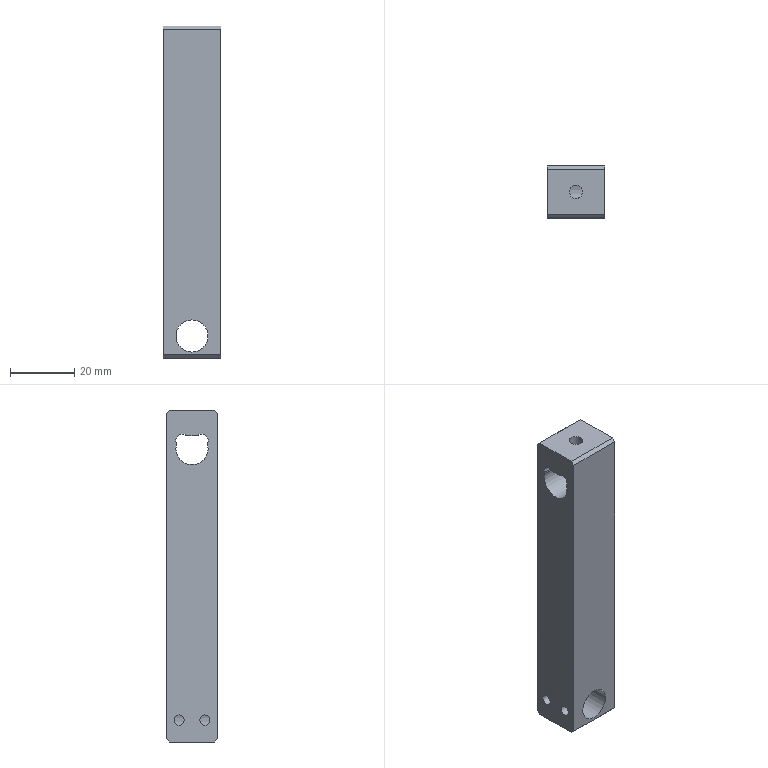Part | NX | 1 solid | 21 faces | box 18 x 16 x 103.264 mm | volume 26814 mm3 | plane 12 | cylinder 9 | commonest cylinder face diameters 2 x2 3.2 x2 4 x2 4.2 x1 10 x1 10.06 x1
STEP:
#1=CARTESIAN_POINT('',(459.468,158.943,-78.23));
#2=VERTEX_POINT('',#1);
#3=CARTESIAN_POINT('',(459.333,160.197,-77.883));
#4=CARTESIAN_POINT('',(459.536,158.943,-78.403));
#5=CARTESIAN_POINT('',(459.333,157.689,-77.883));
#6=CARTESIAN_POINT('',(459.141,157.17,-76.632));
#7=CARTESIAN_POINT('',(459.334,157.69,-75.375));
#8=CARTESIAN_POINT('',(459.536,158.942,-74.857));
#9=CARTESIAN_POINT('',(459.334,160.196,-75.375));
#10=CARTESIAN_POINT('',(459.141,160.716,-76.63));
#11=CARTESIAN_POINT('',(459.333,160.197,-77.883));
#12=CARTESIAN_POINT('',(459.536,158.943,-78.403));
#13=CARTESIAN_POINT('',(459.333,157.689,-77.883));
#14=B_SPLINE_CURVE_WITH_KNOTS('',3,(#3,#4,#5,#6,#7,#8,#9,#10,#11,#12,#13),.UNSPECIFIED.,.T.,.F.,(1,1,1,1,1,1,1,1,1,1,1,1,1,1,1),(-0.003776,-0.002517,-0.001259,0.,0.001259,0.002517,0.003776,0.005035,0.006294,0.007552,0.008811,0.01007,0.01133,0.01259,0.01385),.UNSPECIFIED.);
#15=EDGE_CURVE('',#2,#2,#14,.T.);
#16=ORIENTED_EDGE('',*,*,#15,.T.);
#17=EDGE_LOOP('',(#16));
#18=FACE_BOUND('',#17,.T.);
#19=CARTESIAN_POINT('',(459.468,166.943,-78.23));
#20=VERTEX_POINT('',#19);
#21=CARTESIAN_POINT('',(459.333,168.197,-77.883));
#22=CARTESIAN_POINT('',(459.536,166.943,-78.403));
#23=CARTESIAN_POINT('',(459.333,165.689,-77.883));
#24=CARTESIAN_POINT('',(459.141,165.17,-76.632));
#25=CARTESIAN_POINT('',(459.334,165.69,-75.375));
#26=CARTESIAN_POINT('',(459.536,166.942,-74.857));
#27=CARTESIAN_POINT('',(459.334,168.196,-75.375));
#28=CARTESIAN_POINT('',(459.141,168.716,-76.63));
#29=CARTESIAN_POINT('',(459.333,168.197,-77.883));
#30=CARTESIAN_POINT('',(459.536,166.943,-78.403));
#31=CARTESIAN_POINT('',(459.333,165.689,-77.883));
#32=B_SPLINE_CURVE_WITH_KNOTS('',3,(#21,#22,#23,#24,#25,#26,#27,#28,#29,#30,#31),.UNSPECIFIED.,.T.,.F.,(1,1,1,1,1,1,1,1,1,1,1,1,1,1,1),(-0.003776,-0.002517,-0.001259,0.,0.001259,0.002517,0.003776,0.005035,0.006294,0.007552,0.008811,0.01007,0.01133,0.01259,0.01385),.UNSPECIFIED.);
#33=EDGE_CURVE('',#20,#20,#32,.T.);
#34=ORIENTED_EDGE('',*,*,#33,.T.);
#35=EDGE_LOOP('',(#34));
#36=FACE_BOUND('',#35,.T.);
#37=CARTESIAN_POINT('',(464.205,170.943,-71.63));
#38=VERTEX_POINT('',#37);
#39=CARTESIAN_POINT('',(464.205,170.943,-76.63));
#40=DIRECTION('',(0.,-1.,0.));
#41=DIRECTION('',(0.,0.,1.));
#42=AXIS2_PLACEMENT_3D('',#39,#40,#41);
#43=CIRCLE('',#42,5.);
#44=EDGE_CURVE('',#38,#38,#43,.T.);
#45=ORIENTED_EDGE('',*,*,#44,.F.);
#46=EDGE_LOOP('',(#45));
#47=FACE_BOUND('',#46,.T.);
#48=CARTESIAN_POINT('',(464.205,154.943,-81.63));
#49=VERTEX_POINT('',#48);
#50=CARTESIAN_POINT('',(464.205,154.943,-76.63));
#51=DIRECTION('',(0.,1.,0.));
#52=DIRECTION('',(0.,0.,-1.));
#53=AXIS2_PLACEMENT_3D('',#50,#51,#52);
#54=CIRCLE('',#53,5.);
#55=EDGE_CURVE('',#49,#49,#54,.T.);
#56=ORIENTED_EDGE('',*,*,#55,.F.);
#57=EDGE_LOOP('',(#56));
#58=FACE_BOUND('',#57,.T.);
#59=CARTESIAN_POINT('',(464.205,146.443,-76.63));
#60=DIRECTION('',(0.,-1.,0.));
#61=DIRECTION('',(0.,0.,-1.));
#62=AXIS2_PLACEMENT_3D('',#59,#60,#61);
#63=CYLINDRICAL_SURFACE('',#62,5.);
#64=ADVANCED_FACE('',(#18,#36,#47,#58),#63,.F.);
#65=CARTESIAN_POINT('',(455.205,169.943,-83.464));
#66=VERTEX_POINT('',#65);
#67=CARTESIAN_POINT('',(455.205,170.943,-82.464));
#68=VERTEX_POINT('',#67);
#69=CARTESIAN_POINT('',(455.205,211.443,-41.964));
#70=DIRECTION('',(0.,0.7071,0.7071));
#71=VECTOR('',#70,1000.);
#72=LINE('',#69,#71);
#73=EDGE_CURVE('',#66,#68,#72,.T.);
#74=ORIENTED_EDGE('',*,*,#73,.T.);
#75=CARTESIAN_POINT('',(473.205,170.943,-82.464));
#76=VERTEX_POINT('',#75);
#77=CARTESIAN_POINT('',(466.205,170.943,-82.464));
#78=DIRECTION('',(1.,0.,0.));
#79=VECTOR('',#78,1000.);
#80=LINE('',#77,#79);
#81=EDGE_CURVE('',#68,#76,#80,.T.);
#82=ORIENTED_EDGE('',*,*,#81,.T.);
#83=CARTESIAN_POINT('',(473.205,169.943,-83.464));
#84=VERTEX_POINT('',#83);
#85=CARTESIAN_POINT('',(473.205,211.443,-41.964));
#86=DIRECTION('',(0.,-0.7071,-0.7071));
#87=VECTOR('',#86,1000.);
#88=LINE('',#85,#87);
#89=EDGE_CURVE('',#76,#84,#88,.T.);
#90=ORIENTED_EDGE('',*,*,#89,.T.);
#91=CARTESIAN_POINT('',(466.205,169.943,-83.464));
#92=DIRECTION('',(-1.,0.,0.));
#93=VECTOR('',#92,1000.);
#94=LINE('',#91,#93);
#95=EDGE_CURVE('',#84,#66,#94,.T.);
#96=ORIENTED_EDGE('',*,*,#95,.T.);
#97=EDGE_LOOP('',(#74,#82,#90,#96));
#98=FACE_BOUND('',#97,.T.);
#99=CARTESIAN_POINT('',(466.205,170.943,-82.464));
#100=DIRECTION('',(0.,-0.7071,0.7071));
#101=DIRECTION('',(1.,0.,0.));
#102=AXIS2_PLACEMENT_3D('',#99,#100,#101);
#103=PLANE('',#102);
#104=ADVANCED_FACE('',(#98),#103,.F.);
#105=CARTESIAN_POINT('',(473.205,155.943,-83.464));
#106=VERTEX_POINT('',#105);
#107=CARTESIAN_POINT('',(473.205,154.943,-82.464));
#108=VERTEX_POINT('',#107);
#109=CARTESIAN_POINT('',(473.205,114.443,-41.964));
#110=DIRECTION('',(0.,-0.7071,0.7071));
#111=VECTOR('',#110,1000.);
#112=LINE('',#109,#111);
#113=EDGE_CURVE('',#106,#108,#112,.T.);
#114=ORIENTED_EDGE('',*,*,#113,.T.);
#115=CARTESIAN_POINT('',(455.205,154.943,-82.464));
#116=VERTEX_POINT('',#115);
#117=CARTESIAN_POINT('',(466.205,154.943,-82.464));
#118=DIRECTION('',(-1.,0.,0.));
#119=VECTOR('',#118,1000.);
#120=LINE('',#117,#119);
#121=EDGE_CURVE('',#108,#116,#120,.T.);
#122=ORIENTED_EDGE('',*,*,#121,.T.);
#123=CARTESIAN_POINT('',(455.205,155.943,-83.464));
#124=VERTEX_POINT('',#123);
#125=CARTESIAN_POINT('',(455.205,114.443,-41.964));
#126=DIRECTION('',(0.,0.7071,-0.7071));
#127=VECTOR('',#126,1000.);
#128=LINE('',#125,#127);
#129=EDGE_CURVE('',#116,#124,#128,.T.);
#130=ORIENTED_EDGE('',*,*,#129,.T.);
#131=CARTESIAN_POINT('',(466.205,155.943,-83.464));
#132=DIRECTION('',(1.,0.,0.));
#133=VECTOR('',#132,1000.);
#134=LINE('',#131,#133);
#135=EDGE_CURVE('',#124,#106,#134,.T.);
#136=ORIENTED_EDGE('',*,*,#135,.T.);
#137=EDGE_LOOP('',(#114,#122,#130,#136));
#138=FACE_BOUND('',#137,.T.);
#139=CARTESIAN_POINT('',(466.205,154.943,-82.464));
#140=DIRECTION('',(0.,0.7071,0.7071));
#141=DIRECTION('',(-1.,0.,0.));
#142=AXIS2_PLACEMENT_3D('',#139,#140,#141);
#143=PLANE('',#142);
#144=ADVANCED_FACE('',(#138),#143,.F.);
#145=CARTESIAN_POINT('',(455.205,158.943,-78.23));
#146=VERTEX_POINT('',#145);
#147=CARTESIAN_POINT('',(455.205,158.943,-76.63));
#148=DIRECTION('',(1.,0.,0.));
#149=DIRECTION('',(0.,0.,-1.));
#150=AXIS2_PLACEMENT_3D('',#147,#148,#149);
#151=CIRCLE('',#150,1.6);
#152=EDGE_CURVE('',#146,#146,#151,.T.);
#153=ORIENTED_EDGE('',*,*,#152,.F.);
#154=EDGE_LOOP('',(#153));
#155=FACE_BOUND('',#154,.T.);
#156=ORIENTED_EDGE('',*,*,#15,.F.);
#157=EDGE_LOOP('',(#156));
#158=FACE_BOUND('',#157,.T.);
#159=CARTESIAN_POINT('',(464.205,158.943,-76.63));
#160=DIRECTION('',(-1.,0.,0.));
#161=DIRECTION('',(0.,0.,-1.));
#162=AXIS2_PLACEMENT_3D('',#159,#160,#161);
#163=CYLINDRICAL_SURFACE('',#162,1.6);
#164=ADVANCED_FACE('',(#155,#158),#163,.F.);
#165=CARTESIAN_POINT('',(455.205,166.943,-78.23));
#166=VERTEX_POINT('',#165);
#167=CARTESIAN_POINT('',(455.205,166.943,-76.63));
#168=DIRECTION('',(1.,0.,0.));
#169=DIRECTION('',(0.,0.,-1.));
#170=AXIS2_PLACEMENT_3D('',#167,#168,#169);
#171=CIRCLE('',#170,1.6);
#172=EDGE_CURVE('',#166,#166,#171,.T.);
#173=ORIENTED_EDGE('',*,*,#172,.F.);
#174=EDGE_LOOP('',(#173));
#175=FACE_BOUND('',#174,.T.);
#176=ORIENTED_EDGE('',*,*,#33,.F.);
#177=EDGE_LOOP('',(#176));
#178=FACE_BOUND('',#177,.T.);
#179=CARTESIAN_POINT('',(464.205,166.943,-76.63));
#180=DIRECTION('',(-1.,0.,0.));
#181=DIRECTION('',(0.,0.,-1.));
#182=AXIS2_PLACEMENT_3D('',#179,#180,#181);
#183=CYLINDRICAL_SURFACE('',#182,1.6);
#184=ADVANCED_FACE('',(#175,#178),#183,.F.);
#185=CARTESIAN_POINT('',(473.205,162.943,-83.464));
#186=DIRECTION('',(0.,-1.,0.));
#187=VECTOR('',#186,1000.);
#188=LINE('',#185,#187);
#189=EDGE_CURVE('',#84,#106,#188,.T.);
#190=ORIENTED_EDGE('',*,*,#189,.T.);
#191=ORIENTED_EDGE('',*,*,#135,.F.);
#192=CARTESIAN_POINT('',(455.205,162.943,-83.464));
#193=DIRECTION('',(0.,1.,0.));
#194=VECTOR('',#193,1000.);
#195=LINE('',#192,#194);
#196=EDGE_CURVE('',#124,#66,#195,.T.);
#197=ORIENTED_EDGE('',*,*,#196,.T.);
#198=ORIENTED_EDGE('',*,*,#95,.F.);
#199=EDGE_LOOP('',(#190,#191,#197,#198));
#200=FACE_BOUND('',#199,.T.);
#201=CARTESIAN_POINT('',(466.205,162.943,-83.464));
#202=DIRECTION('',(0.,0.,-1.));
#203=DIRECTION('',(1.,0.,0.));
#204=AXIS2_PLACEMENT_3D('',#201,#202,#203);
#205=PLANE('',#204);
#206=ADVANCED_FACE('',(#200),#205,.T.);
#207=CARTESIAN_POINT('',(455.205,167.836,9.657));
#208=VERTEX_POINT('',#207);
#209=CARTESIAN_POINT('',(455.205,164.63,11.83));
#210=VERTEX_POINT('',#209);
#211=CARTESIAN_POINT('',(455.205,165.953,10.33));
#212=DIRECTION('',(1.,0.,0.));
#213=DIRECTION('',(0.,0.,-1.));
#214=AXIS2_PLACEMENT_3D('',#211,#212,#213);
#215=CIRCLE('',#214,2.);
#216=EDGE_CURVE('',#208,#210,#215,.T.);
#217=ORIENTED_EDGE('',*,*,#216,.F.);
#218=CARTESIAN_POINT('',(473.205,167.836,9.657));
#219=VERTEX_POINT('',#218);
#220=CARTESIAN_POINT('',(473.205,167.836,9.657));
#221=DIRECTION('',(-1.,0.,0.));
#222=VECTOR('',#221,1000.);
#223=LINE('',#220,#222);
#224=EDGE_CURVE('',#208,#219,#223,.F.);
#225=ORIENTED_EDGE('',*,*,#224,.T.);
#226=CARTESIAN_POINT('',(473.205,164.63,11.83));
#227=VERTEX_POINT('',#226);
#228=CARTESIAN_POINT('',(473.205,165.953,10.33));
#229=DIRECTION('',(1.,0.,0.));
#230=DIRECTION('',(0.,0.,-1.));
#231=AXIS2_PLACEMENT_3D('',#228,#229,#230);
#232=CIRCLE('',#231,2.);
#233=EDGE_CURVE('',#219,#227,#232,.T.);
#234=ORIENTED_EDGE('',*,*,#233,.T.);
#235=CARTESIAN_POINT('',(465.456,164.63,11.83));
#236=VERTEX_POINT('',#235);
#237=CARTESIAN_POINT('',(473.205,164.63,11.83));
#238=DIRECTION('',(-1.,0.,0.));
#239=VECTOR('',#238,1000.);
#240=LINE('',#237,#239);
#241=EDGE_CURVE('',#227,#236,#240,.T.);
#242=ORIENTED_EDGE('',*,*,#241,.T.);
#243=CARTESIAN_POINT('',(462.955,164.63,11.83));
#244=VERTEX_POINT('',#243);
#245=CARTESIAN_POINT('',(465.456,164.63,11.83));
#246=CARTESIAN_POINT('',(465.125,164.875,12.046));
#247=CARTESIAN_POINT('',(464.206,165.211,12.176));
#248=CARTESIAN_POINT('',(463.286,164.875,12.046));
#249=CARTESIAN_POINT('',(462.955,164.63,11.83));
#250=B_SPLINE_CURVE_WITH_KNOTS('',3,(#245,#246,#247,#248,#249),.UNSPECIFIED.,.F.,.F.,(4,1,4),(0.,0.001373,0.002746),.UNSPECIFIED.);
#251=EDGE_CURVE('',#236,#244,#250,.T.);
#252=ORIENTED_EDGE('',*,*,#251,.T.);
#253=CARTESIAN_POINT('',(473.205,164.63,11.83));
#254=DIRECTION('',(-1.,0.,0.));
#255=VECTOR('',#254,1000.);
#256=LINE('',#253,#255);
#257=EDGE_CURVE('',#244,#210,#256,.T.);
#258=ORIENTED_EDGE('',*,*,#257,.T.);
#259=EDGE_LOOP('',(#217,#225,#234,#242,#252,#258));
#260=FACE_BOUND('',#259,.T.);
#261=CARTESIAN_POINT('',(473.205,165.953,10.33));
#262=DIRECTION('',(-1.,0.,0.));
#263=DIRECTION('',(0.,0.,-1.));
#264=AXIS2_PLACEMENT_3D('',#261,#262,#263);
#265=CYLINDRICAL_SURFACE('',#264,2.);
#266=ADVANCED_FACE('',(#260),#265,.F.);
#267=CARTESIAN_POINT('',(473.205,161.256,11.83));
#268=VERTEX_POINT('',#267);
#269=CARTESIAN_POINT('',(473.205,158.05,9.657));
#270=VERTEX_POINT('',#269);
#271=CARTESIAN_POINT('',(473.205,159.933,10.33));
#272=DIRECTION('',(1.,0.,0.));
#273=DIRECTION('',(0.,0.,-1.));
#274=AXIS2_PLACEMENT_3D('',#271,#272,#273);
#275=CIRCLE('',#274,2.);
#276=EDGE_CURVE('',#268,#270,#275,.T.);
#277=ORIENTED_EDGE('',*,*,#276,.T.);
#278=CARTESIAN_POINT('',(455.205,158.05,9.657));
#279=VERTEX_POINT('',#278);
#280=CARTESIAN_POINT('',(473.205,158.05,9.657));
#281=DIRECTION('',(-1.,0.,0.));
#282=VECTOR('',#281,1000.);
#283=LINE('',#280,#282);
#284=EDGE_CURVE('',#270,#279,#283,.T.);
#285=ORIENTED_EDGE('',*,*,#284,.T.);
#286=CARTESIAN_POINT('',(455.205,161.256,11.83));
#287=VERTEX_POINT('',#286);
#288=CARTESIAN_POINT('',(455.205,159.933,10.33));
#289=DIRECTION('',(1.,0.,0.));
#290=DIRECTION('',(0.,0.,-1.));
#291=AXIS2_PLACEMENT_3D('',#288,#289,#290);
#292=CIRCLE('',#291,2.);
#293=EDGE_CURVE('',#287,#279,#292,.T.);
#294=ORIENTED_EDGE('',*,*,#293,.F.);
#295=CARTESIAN_POINT('',(462.955,161.256,11.83));
#296=VERTEX_POINT('',#295);
#297=CARTESIAN_POINT('',(473.205,161.256,11.83));
#298=DIRECTION('',(1.,0.,0.));
#299=VECTOR('',#298,1000.);
#300=LINE('',#297,#299);
#301=EDGE_CURVE('',#287,#296,#300,.T.);
#302=ORIENTED_EDGE('',*,*,#301,.T.);
#303=CARTESIAN_POINT('',(465.456,161.256,11.83));
#304=VERTEX_POINT('',#303);
#305=CARTESIAN_POINT('',(462.955,161.256,11.83));
#306=CARTESIAN_POINT('',(463.286,161.011,12.046));
#307=CARTESIAN_POINT('',(464.205,160.675,12.176));
#308=CARTESIAN_POINT('',(465.125,161.011,12.046));
#309=CARTESIAN_POINT('',(465.456,161.256,11.83));
#310=B_SPLINE_CURVE_WITH_KNOTS('',3,(#305,#306,#307,#308,#309),.UNSPECIFIED.,.F.,.F.,(4,1,4),(0.,0.001373,0.002746),.UNSPECIFIED.);
#311=EDGE_CURVE('',#296,#304,#310,.T.);
#312=ORIENTED_EDGE('',*,*,#311,.T.);
#313=CARTESIAN_POINT('',(473.205,161.256,11.83));
#314=DIRECTION('',(1.,0.,0.));
#315=VECTOR('',#314,1000.);
#316=LINE('',#313,#315);
#317=EDGE_CURVE('',#304,#268,#316,.T.);
#318=ORIENTED_EDGE('',*,*,#317,.T.);
#319=EDGE_LOOP('',(#277,#285,#294,#302,#312,#318));
#320=FACE_BOUND('',#319,.T.);
#321=CARTESIAN_POINT('',(473.205,159.933,10.33));
#322=DIRECTION('',(-1.,0.,0.));
#323=DIRECTION('',(0.,0.,-1.));
#324=AXIS2_PLACEMENT_3D('',#321,#322,#323);
#325=CYLINDRICAL_SURFACE('',#324,2.);
#326=ADVANCED_FACE('',(#320),#325,.F.);
#327=CARTESIAN_POINT('',(455.205,155.943,19.8));
#328=VERTEX_POINT('',#327);
#329=CARTESIAN_POINT('',(455.205,154.943,18.8));
#330=VERTEX_POINT('',#329);
#331=CARTESIAN_POINT('',(455.205,149.943,13.8));
#332=DIRECTION('',(0.,-0.7071,-0.7071));
#333=VECTOR('',#332,1000.);
#334=LINE('',#331,#333);
#335=EDGE_CURVE('',#328,#330,#334,.T.);
#336=ORIENTED_EDGE('',*,*,#335,.T.);
#337=CARTESIAN_POINT('',(473.205,154.943,18.8));
#338=VERTEX_POINT('',#337);
#339=CARTESIAN_POINT('',(466.205,154.943,18.8));
#340=DIRECTION('',(1.,0.,0.));
#341=VECTOR('',#340,1000.);
#342=LINE('',#339,#341);
#343=EDGE_CURVE('',#330,#338,#342,.T.);
#344=ORIENTED_EDGE('',*,*,#343,.T.);
#345=CARTESIAN_POINT('',(473.205,155.943,19.8));
#346=VERTEX_POINT('',#345);
#347=CARTESIAN_POINT('',(473.205,149.943,13.8));
#348=DIRECTION('',(0.,0.7071,0.7071));
#349=VECTOR('',#348,1000.);
#350=LINE('',#347,#349);
#351=EDGE_CURVE('',#338,#346,#350,.T.);
#352=ORIENTED_EDGE('',*,*,#351,.T.);
#353=CARTESIAN_POINT('',(466.205,155.943,19.8));
#354=DIRECTION('',(-1.,0.,0.));
#355=VECTOR('',#354,1000.);
#356=LINE('',#353,#355);
#357=EDGE_CURVE('',#346,#328,#356,.T.);
#358=ORIENTED_EDGE('',*,*,#357,.T.);
#359=EDGE_LOOP('',(#336,#344,#352,#358));
#360=FACE_BOUND('',#359,.T.);
#361=CARTESIAN_POINT('',(466.205,154.943,18.8));
#362=DIRECTION('',(0.,0.7071,-0.7071));
#363=DIRECTION('',(1.,0.,0.));
#364=AXIS2_PLACEMENT_3D('',#361,#362,#363);
#365=PLANE('',#364);
#366=ADVANCED_FACE('',(#360),#365,.F.);
#367=CARTESIAN_POINT('',(473.205,169.943,19.8));
#368=VERTEX_POINT('',#367);
#369=CARTESIAN_POINT('',(473.205,170.943,18.8));
#370=VERTEX_POINT('',#369);
#371=CARTESIAN_POINT('',(473.205,175.943,13.8));
#372=DIRECTION('',(0.,0.7071,-0.7071));
#373=VECTOR('',#372,1000.);
#374=LINE('',#371,#373);
#375=EDGE_CURVE('',#368,#370,#374,.T.);
#376=ORIENTED_EDGE('',*,*,#375,.T.);
#377=CARTESIAN_POINT('',(455.205,170.943,18.8));
#378=VERTEX_POINT('',#377);
#379=CARTESIAN_POINT('',(466.205,170.943,18.8));
#380=DIRECTION('',(-1.,0.,0.));
#381=VECTOR('',#380,1000.);
#382=LINE('',#379,#381);
#383=EDGE_CURVE('',#370,#378,#382,.T.);
#384=ORIENTED_EDGE('',*,*,#383,.T.);
#385=CARTESIAN_POINT('',(455.205,169.943,19.8));
#386=VERTEX_POINT('',#385);
#387=CARTESIAN_POINT('',(455.205,175.943,13.8));
#388=DIRECTION('',(0.,-0.7071,0.7071));
#389=VECTOR('',#388,1000.);
#390=LINE('',#387,#389);
#391=EDGE_CURVE('',#378,#386,#390,.T.);
#392=ORIENTED_EDGE('',*,*,#391,.T.);
#393=CARTESIAN_POINT('',(466.205,169.943,19.8));
#394=DIRECTION('',(1.,0.,0.));
#395=VECTOR('',#394,1000.);
#396=LINE('',#393,#395);
#397=EDGE_CURVE('',#386,#368,#396,.T.);
#398=ORIENTED_EDGE('',*,*,#397,.T.);
#399=EDGE_LOOP('',(#376,#384,#392,#398));
#400=FACE_BOUND('',#399,.T.);
#401=CARTESIAN_POINT('',(466.205,170.943,18.8));
#402=DIRECTION('',(0.,-0.7071,-0.7071));
#403=DIRECTION('',(-1.,0.,0.));
#404=AXIS2_PLACEMENT_3D('',#401,#402,#403);
#405=PLANE('',#404);
#406=ADVANCED_FACE('',(#400),#405,.F.);
#407=CARTESIAN_POINT('',(464.205,162.943,11.83));
#408=DIRECTION('',(0.,0.,-1.));
#409=DIRECTION('',(-1.,0.,0.));
#410=AXIS2_PLACEMENT_3D('',#407,#408,#409);
#411=CIRCLE('',#410,2.1);
#412=EDGE_CURVE('',#236,#304,#411,.T.);
#413=ORIENTED_EDGE('',*,*,#412,.T.);
#414=ORIENTED_EDGE('',*,*,#311,.F.);
#415=CARTESIAN_POINT('',(464.205,162.943,11.83));
#416=DIRECTION('',(0.,0.,-1.));
#417=DIRECTION('',(-1.,0.,0.));
#418=AXIS2_PLACEMENT_3D('',#415,#416,#417);
#419=CIRCLE('',#418,2.1);
#420=EDGE_CURVE('',#296,#244,#419,.T.);
#421=ORIENTED_EDGE('',*,*,#420,.T.);
#422=ORIENTED_EDGE('',*,*,#251,.F.);
#423=EDGE_LOOP('',(#413,#414,#421,#422));
#424=FACE_BOUND('',#423,.T.);
#425=CARTESIAN_POINT('',(462.105,162.943,19.8));
#426=VERTEX_POINT('',#425);
#427=CARTESIAN_POINT('',(464.205,162.943,19.8));
#428=DIRECTION('',(0.,0.,1.));
#429=DIRECTION('',(-1.,0.,0.));
#430=AXIS2_PLACEMENT_3D('',#427,#428,#429);
#431=CIRCLE('',#430,2.1);
#432=EDGE_CURVE('',#426,#426,#431,.T.);
#433=ORIENTED_EDGE('',*,*,#432,.T.);
#434=EDGE_LOOP('',(#433));
#435=FACE_BOUND('',#434,.T.);
#436=CARTESIAN_POINT('',(464.205,162.943,19.8));
#437=DIRECTION('',(0.,0.,-1.));
#438=DIRECTION('',(-1.,0.,0.));
#439=AXIS2_PLACEMENT_3D('',#436,#437,#438);
#440=CYLINDRICAL_SURFACE('',#439,2.1);
#441=ADVANCED_FACE('',(#424,#435),#440,.F.);
#442=ORIENTED_EDGE('',*,*,#420,.F.);
#443=ORIENTED_EDGE('',*,*,#301,.F.);
#444=CARTESIAN_POINT('',(455.205,162.943,11.83));
#445=DIRECTION('',(0.,-1.,0.));
#446=VECTOR('',#445,1000.);
#447=LINE('',#444,#446);
#448=EDGE_CURVE('',#210,#287,#447,.T.);
#449=ORIENTED_EDGE('',*,*,#448,.F.);
#450=ORIENTED_EDGE('',*,*,#257,.F.);
#451=EDGE_LOOP('',(#442,#443,#449,#450));
#452=FACE_BOUND('',#451,.T.);
#453=CARTESIAN_POINT('',(488.102,129.943,11.83));
#454=DIRECTION('',(0.,0.,1.));
#455=DIRECTION('',(-1.,0.,0.));
#456=AXIS2_PLACEMENT_3D('',#453,#454,#455);
#457=PLANE('',#456);
#458=ADVANCED_FACE('',(#452),#457,.F.);
#459=CARTESIAN_POINT('',(455.205,167.81,9.069));
#460=VERTEX_POINT('',#459);
#461=CARTESIAN_POINT('',(455.205,158.076,9.069));
#462=VERTEX_POINT('',#461);
#463=CARTESIAN_POINT('',(455.205,162.943,7.8));
#464=DIRECTION('',(-1.,0.,0.));
#465=DIRECTION('',(0.,0.,-1.));
#466=AXIS2_PLACEMENT_3D('',#463,#464,#465);
#467=CIRCLE('',#466,5.03);
#468=EDGE_CURVE('',#460,#462,#467,.T.);
#469=ORIENTED_EDGE('',*,*,#468,.T.);
#470=CARTESIAN_POINT('',(473.205,158.076,9.069));
#471=VERTEX_POINT('',#470);
#472=CARTESIAN_POINT('',(512.602,158.076,9.069));
#473=DIRECTION('',(-1.,0.,0.));
#474=VECTOR('',#473,1000.);
#475=LINE('',#472,#474);
#476=EDGE_CURVE('',#462,#471,#475,.F.);
#477=ORIENTED_EDGE('',*,*,#476,.T.);
#478=CARTESIAN_POINT('',(473.205,167.81,9.069));
#479=VERTEX_POINT('',#478);
#480=CARTESIAN_POINT('',(473.205,162.943,7.8));
#481=DIRECTION('',(1.,0.,0.));
#482=DIRECTION('',(0.,0.,1.));
#483=AXIS2_PLACEMENT_3D('',#480,#481,#482);
#484=CIRCLE('',#483,5.03);
#485=EDGE_CURVE('',#471,#479,#484,.T.);
#486=ORIENTED_EDGE('',*,*,#485,.T.);
#487=CARTESIAN_POINT('',(512.602,167.81,9.069));
#488=DIRECTION('',(-1.,0.,0.));
#489=VECTOR('',#488,1000.);
#490=LINE('',#487,#489);
#491=EDGE_CURVE('',#479,#460,#490,.T.);
#492=ORIENTED_EDGE('',*,*,#491,.T.);
#493=EDGE_LOOP('',(#469,#477,#486,#492));
#494=FACE_BOUND('',#493,.T.);
#495=CARTESIAN_POINT('',(512.602,162.943,7.8));
#496=DIRECTION('',(-1.,0.,0.));
#497=DIRECTION('',(0.,0.,1.));
#498=AXIS2_PLACEMENT_3D('',#495,#496,#497);
#499=CYLINDRICAL_SURFACE('',#498,5.03);
#500=ADVANCED_FACE('',(#494),#499,.F.);
#501=ORIENTED_EDGE('',*,*,#44,.T.);
#502=EDGE_LOOP('',(#501));
#503=FACE_BOUND('',#502,.T.);
#504=CARTESIAN_POINT('',(455.205,170.943,0.8));
#505=DIRECTION('',(0.,0.,1.));
#506=VECTOR('',#505,1000.);
#507=LINE('',#504,#506);
#508=EDGE_CURVE('',#68,#378,#507,.T.);
#509=ORIENTED_EDGE('',*,*,#508,.T.);
#510=ORIENTED_EDGE('',*,*,#383,.F.);
#511=CARTESIAN_POINT('',(473.205,170.943,0.8));
#512=DIRECTION('',(0.,0.,1.));
#513=VECTOR('',#512,1000.);
#514=LINE('',#511,#513);
#515=EDGE_CURVE('',#76,#370,#514,.T.);
#516=ORIENTED_EDGE('',*,*,#515,.F.);
#517=ORIENTED_EDGE('',*,*,#81,.F.);
#518=EDGE_LOOP('',(#509,#510,#516,#517));
#519=FACE_BOUND('',#518,.T.);
#520=CARTESIAN_POINT('',(466.205,170.943,0.8));
#521=DIRECTION('',(0.,1.,0.));
#522=DIRECTION('',(0.,0.,1.));
#523=AXIS2_PLACEMENT_3D('',#520,#521,#522);
#524=PLANE('',#523);
#525=ADVANCED_FACE('',(#503,#519),#524,.T.);
#526=ORIENTED_EDGE('',*,*,#55,.T.);
#527=EDGE_LOOP('',(#526));
#528=FACE_BOUND('',#527,.T.);
#529=CARTESIAN_POINT('',(473.205,154.943,0.8));
#530=DIRECTION('',(0.,0.,1.));
#531=VECTOR('',#530,1000.);
#532=LINE('',#529,#531);
#533=EDGE_CURVE('',#108,#338,#532,.T.);
#534=ORIENTED_EDGE('',*,*,#533,.T.);
#535=ORIENTED_EDGE('',*,*,#343,.F.);
#536=CARTESIAN_POINT('',(455.205,154.943,0.8));
#537=DIRECTION('',(0.,0.,1.));
#538=VECTOR('',#537,1000.);
#539=LINE('',#536,#538);
#540=EDGE_CURVE('',#116,#330,#539,.T.);
#541=ORIENTED_EDGE('',*,*,#540,.F.);
#542=ORIENTED_EDGE('',*,*,#121,.F.);
#543=EDGE_LOOP('',(#534,#535,#541,#542));
#544=FACE_BOUND('',#543,.T.);
#545=CARTESIAN_POINT('',(466.205,154.943,0.8));
#546=DIRECTION('',(0.,-1.,0.));
#547=DIRECTION('',(0.,0.,-1.));
#548=AXIS2_PLACEMENT_3D('',#545,#546,#547);
#549=PLANE('',#548);
#550=ADVANCED_FACE('',(#528,#544),#549,.T.);
#551=CARTESIAN_POINT('',(455.205,162.943,19.8));
#552=DIRECTION('',(0.,-1.,0.));
#553=VECTOR('',#552,1000.);
#554=LINE('',#551,#553);
#555=EDGE_CURVE('',#386,#328,#554,.T.);
#556=ORIENTED_EDGE('',*,*,#555,.T.);
#557=ORIENTED_EDGE('',*,*,#357,.F.);
#558=CARTESIAN_POINT('',(473.205,162.943,19.8));
#559=DIRECTION('',(0.,1.,0.));
#560=VECTOR('',#559,1000.);
#561=LINE('',#558,#560);
#562=EDGE_CURVE('',#346,#368,#561,.T.);
#563=ORIENTED_EDGE('',*,*,#562,.T.);
#564=ORIENTED_EDGE('',*,*,#397,.F.);
#565=EDGE_LOOP('',(#556,#557,#563,#564));
#566=FACE_BOUND('',#565,.T.);
#567=ORIENTED_EDGE('',*,*,#432,.F.);
#568=EDGE_LOOP('',(#567));
#569=FACE_BOUND('',#568,.T.);
#570=CARTESIAN_POINT('',(466.205,162.943,19.8));
#571=DIRECTION('',(0.,0.,1.));
#572=DIRECTION('',(-1.,0.,0.));
#573=AXIS2_PLACEMENT_3D('',#570,#571,#572);
#574=PLANE('',#573);
#575=ADVANCED_FACE('',(#566,#569),#574,.T.);
#576=ORIENTED_EDGE('',*,*,#172,.T.);
#577=EDGE_LOOP('',(#576));
#578=FACE_BOUND('',#577,.T.);
#579=ORIENTED_EDGE('',*,*,#152,.T.);
#580=EDGE_LOOP('',(#579));
#581=FACE_BOUND('',#580,.T.);
#582=ORIENTED_EDGE('',*,*,#293,.T.);
#583=CARTESIAN_POINT('',(455.205,157.108,9.321));
#584=DIRECTION('',(-1.,0.,0.));
#585=DIRECTION('',(0.,0.,1.));
#586=AXIS2_PLACEMENT_3D('',#583,#584,#585);
#587=CIRCLE('',#586,1.);
#588=EDGE_CURVE('',#279,#462,#587,.T.);
#589=ORIENTED_EDGE('',*,*,#588,.T.);
#590=ORIENTED_EDGE('',*,*,#468,.F.);
#591=CARTESIAN_POINT('',(455.205,168.778,9.321));
#592=DIRECTION('',(-1.,0.,0.));
#593=DIRECTION('',(0.,0.,1.));
#594=AXIS2_PLACEMENT_3D('',#591,#592,#593);
#595=CIRCLE('',#594,1.);
#596=EDGE_CURVE('',#460,#208,#595,.T.);
#597=ORIENTED_EDGE('',*,*,#596,.T.);
#598=ORIENTED_EDGE('',*,*,#216,.T.);
#599=ORIENTED_EDGE('',*,*,#448,.T.);
#600=EDGE_LOOP('',(#582,#589,#590,#597,#598,#599));
#601=FACE_BOUND('',#600,.T.);
#602=ORIENTED_EDGE('',*,*,#540,.T.);
#603=ORIENTED_EDGE('',*,*,#335,.F.);
#604=ORIENTED_EDGE('',*,*,#555,.F.);
#605=ORIENTED_EDGE('',*,*,#391,.F.);
#606=ORIENTED_EDGE('',*,*,#508,.F.);
#607=ORIENTED_EDGE('',*,*,#73,.F.);
#608=ORIENTED_EDGE('',*,*,#196,.F.);
#609=ORIENTED_EDGE('',*,*,#129,.F.);
#610=EDGE_LOOP('',(#602,#603,#604,#605,#606,#607,#608,#609));
#611=FACE_BOUND('',#610,.T.);
#612=CARTESIAN_POINT('',(455.205,162.943,0.8));
#613=DIRECTION('',(-1.,0.,0.));
#614=DIRECTION('',(0.,0.,-1.));
#615=AXIS2_PLACEMENT_3D('',#612,#613,#614);
#616=PLANE('',#615);
#617=ADVANCED_FACE('',(#578,#581,#601,#611),#616,.T.);
#618=CARTESIAN_POINT('',(473.205,162.943,11.83));
#619=DIRECTION('',(0.,1.,0.));
#620=VECTOR('',#619,1000.);
#621=LINE('',#618,#620);
#622=EDGE_CURVE('',#268,#227,#621,.T.);
#623=ORIENTED_EDGE('',*,*,#622,.F.);
#624=ORIENTED_EDGE('',*,*,#317,.F.);
#625=ORIENTED_EDGE('',*,*,#412,.F.);
#626=ORIENTED_EDGE('',*,*,#241,.F.);
#627=EDGE_LOOP('',(#623,#624,#625,#626));
#628=FACE_BOUND('',#627,.T.);
#629=CARTESIAN_POINT('',(488.102,129.943,11.83));
#630=DIRECTION('',(0.,0.,1.));
#631=DIRECTION('',(-1.,0.,0.));
#632=AXIS2_PLACEMENT_3D('',#629,#630,#631);
#633=PLANE('',#632);
#634=ADVANCED_FACE('',(#628),#633,.F.);
#635=ORIENTED_EDGE('',*,*,#485,.F.);
#636=CARTESIAN_POINT('',(473.205,157.108,9.321));
#637=DIRECTION('',(1.,0.,0.));
#638=DIRECTION('',(0.,0.,-1.));
#639=AXIS2_PLACEMENT_3D('',#636,#637,#638);
#640=CIRCLE('',#639,1.);
#641=EDGE_CURVE('',#471,#270,#640,.T.);
#642=ORIENTED_EDGE('',*,*,#641,.T.);
#643=ORIENTED_EDGE('',*,*,#276,.F.);
#644=ORIENTED_EDGE('',*,*,#622,.T.);
#645=ORIENTED_EDGE('',*,*,#233,.F.);
#646=CARTESIAN_POINT('',(473.205,168.778,9.321));
#647=DIRECTION('',(1.,0.,0.));
#648=DIRECTION('',(0.,0.,-1.));
#649=AXIS2_PLACEMENT_3D('',#646,#647,#648);
#650=CIRCLE('',#649,1.);
#651=EDGE_CURVE('',#219,#479,#650,.T.);
#652=ORIENTED_EDGE('',*,*,#651,.T.);
#653=EDGE_LOOP('',(#635,#642,#643,#644,#645,#652));
#654=FACE_BOUND('',#653,.T.);
#655=ORIENTED_EDGE('',*,*,#515,.T.);
#656=ORIENTED_EDGE('',*,*,#375,.F.);
#657=ORIENTED_EDGE('',*,*,#562,.F.);
#658=ORIENTED_EDGE('',*,*,#351,.F.);
#659=ORIENTED_EDGE('',*,*,#533,.F.);
#660=ORIENTED_EDGE('',*,*,#113,.F.);
#661=ORIENTED_EDGE('',*,*,#189,.F.);
#662=ORIENTED_EDGE('',*,*,#89,.F.);
#663=EDGE_LOOP('',(#655,#656,#657,#658,#659,#660,#661,#662));
#664=FACE_BOUND('',#663,.T.);
#665=CARTESIAN_POINT('',(473.205,162.943,0.8));
#666=DIRECTION('',(1.,0.,0.));
#667=DIRECTION('',(0.,0.,1.));
#668=AXIS2_PLACEMENT_3D('',#665,#666,#667);
#669=PLANE('',#668);
#670=ADVANCED_FACE('',(#654,#664),#669,.T.);
#671=ORIENTED_EDGE('',*,*,#588,.F.);
#672=ORIENTED_EDGE('',*,*,#284,.F.);
#673=ORIENTED_EDGE('',*,*,#641,.F.);
#674=ORIENTED_EDGE('',*,*,#476,.F.);
#675=EDGE_LOOP('',(#671,#672,#673,#674));
#676=FACE_BOUND('',#675,.T.);
#677=CARTESIAN_POINT('',(473.205,157.108,9.321));
#678=DIRECTION('',(1.,0.,0.));
#679=DIRECTION('',(0.,0.,-1.));
#680=AXIS2_PLACEMENT_3D('',#677,#678,#679);
#681=CYLINDRICAL_SURFACE('',#680,1.);
#682=ADVANCED_FACE('',(#676),#681,.T.);
#683=ORIENTED_EDGE('',*,*,#651,.F.);
#684=ORIENTED_EDGE('',*,*,#224,.F.);
#685=ORIENTED_EDGE('',*,*,#596,.F.);
#686=ORIENTED_EDGE('',*,*,#491,.F.);
#687=EDGE_LOOP('',(#683,#684,#685,#686));
#688=FACE_BOUND('',#687,.T.);
#689=CARTESIAN_POINT('',(473.205,168.778,9.321));
#690=DIRECTION('',(-1.,0.,0.));
#691=DIRECTION('',(0.,0.,1.));
#692=AXIS2_PLACEMENT_3D('',#689,#690,#691);
#693=CYLINDRICAL_SURFACE('',#692,1.);
#694=ADVANCED_FACE('',(#688),#693,.T.);
#695=CLOSED_SHELL('',(#64,#104,#144,#164,#184,#206,#266,#326,#366,#406,#441,#458,#500,#525,#550,#575,#617,#634,#670,#682,#694));
#696=MANIFOLD_SOLID_BREP('',#695);
#697=(LENGTH_UNIT()NAMED_UNIT(*)SI_UNIT(.MILLI.,.METRE.));
#698=UNCERTAINTY_MEASURE_WITH_UNIT(LENGTH_MEASURE(0.0508),#697,'','');
#699=(NAMED_UNIT(*)PLANE_ANGLE_UNIT()SI_UNIT($,.RADIAN.));
#700=(NAMED_UNIT(*)SI_UNIT($,.STERADIAN.)SOLID_ANGLE_UNIT());
#701=(GEOMETRIC_REPRESENTATION_CONTEXT(3)GLOBAL_UNCERTAINTY_ASSIGNED_CONTEXT((#698))GLOBAL_UNIT_ASSIGNED_CONTEXT((#697,#699,#700))REPRESENTATION_CONTEXT('',''));
#702=ADVANCED_BREP_SHAPE_REPRESENTATION('',(#696),#701);